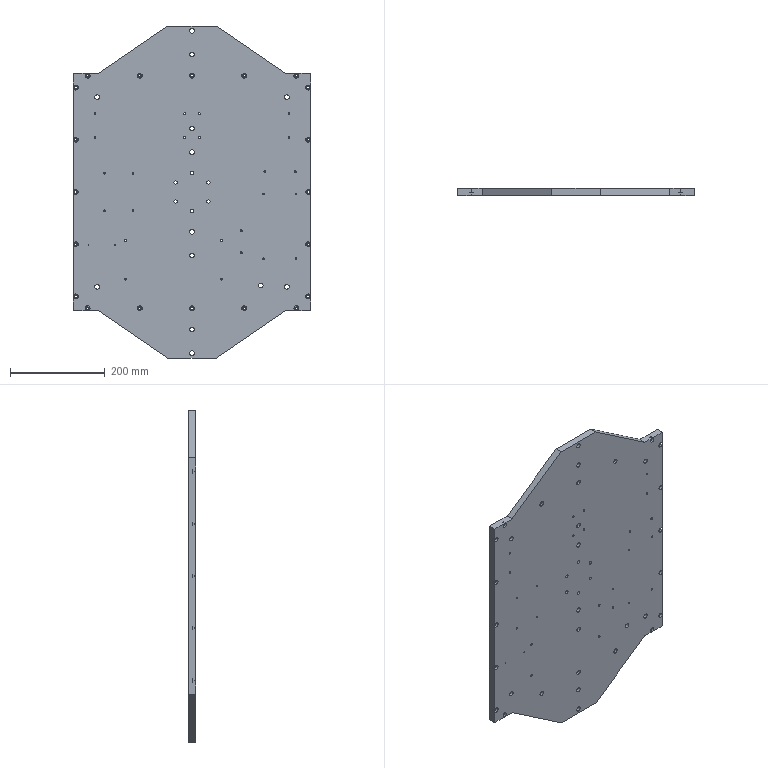Part | 1 solid | 221 faces | box 500 x 15 x 700 mm | volume 4432854 mm3 | cylinder 182 | plane 39 | commonest cylinder face diameters 10.1 x48 5.5 x40 4.2 x32 10.2 x26 3.3 x16 6.8 x12